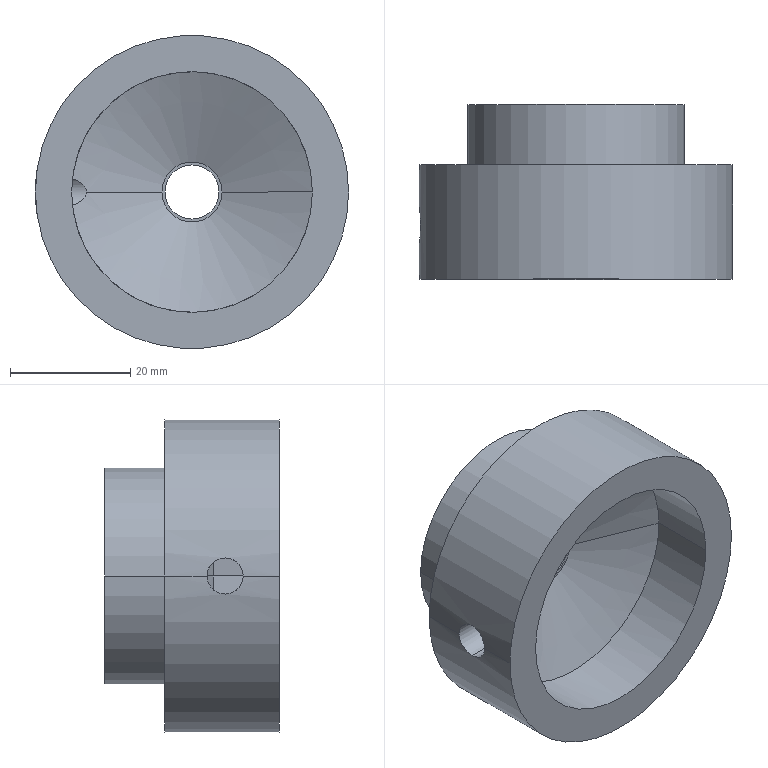Part | SolidWorks | features HoleWzd 1, ICE 1, Revolution 1 | 1 solid | 16 faces | box 52 x 29 x 52 mm | volume 32471 mm3 | cylinder 10 | plane 4 | cone 2 | commonest cylinder face diameters 6 x2 9 x2 36 x2 40 x2 52 x2
STEP:
#1=CARTESIAN_POINT('',(-25.826,9.,3.));
#2=VERTEX_POINT('',#1);
#3=CARTESIAN_POINT('',(-26.,6.,0.));
#4=VERTEX_POINT('',#3);
#5=CARTESIAN_POINT('',(-25.826,9.,3.));
#6=CARTESIAN_POINT('',(-25.826,8.802,3.));
#7=CARTESIAN_POINT('',(-25.829,8.607,2.981));
#8=CARTESIAN_POINT('',(-25.837,8.223,2.904));
#9=CARTESIAN_POINT('',(-25.844,8.033,2.847));
#10=CARTESIAN_POINT('',(-25.86,7.67,2.696));
#11=CARTESIAN_POINT('',(-25.869,7.498,2.604));
#12=CARTESIAN_POINT('',(-25.89,7.172,2.387));
#13=CARTESIAN_POINT('',(-25.902,7.018,2.26));
#14=CARTESIAN_POINT('',(-25.925,6.741,1.984));
#15=CARTESIAN_POINT('',(-25.936,6.617,1.833));
#16=CARTESIAN_POINT('',(-25.957,6.398,1.506));
#17=CARTESIAN_POINT('',(-25.967,6.305,1.331));
#18=CARTESIAN_POINT('',(-25.982,6.155,0.9708));
#19=CARTESIAN_POINT('',(-25.989,6.097,0.7819));
#20=CARTESIAN_POINT('',(-25.998,6.019,0.3943));
#21=CARTESIAN_POINT('',(-26.,6.,0.1983));
#22=CARTESIAN_POINT('',(-26.,6.,0.));
#23=B_SPLINE_CURVE_WITH_KNOTS('',3,(#5,#6,#7,#8,#9,#10,#11,#12,#13,#14,#15,#16,#17,#18,#19,#20,#21,#22),.UNSPECIFIED.,.F.,.F.,(4,2,2,2,2,2,2,2,4),(0.01408,0.01467,0.01525,0.01584,0.01643,0.01701,0.0176,0.01819,0.01877),.UNSPECIFIED.);
#24=EDGE_CURVE('',#2,#4,#23,.T.);
#25=ORIENTED_EDGE('',*,*,#24,.F.);
#26=CARTESIAN_POINT('',(-19.774,9.,3.));
#27=VERTEX_POINT('',#26);
#28=CARTESIAN_POINT('',(-26.,9.,3.));
#29=DIRECTION('',(1.,0.,0.));
#30=VECTOR('',#29,1000.);
#31=LINE('',#28,#30);
#32=EDGE_CURVE('',#2,#27,#31,.T.);
#33=ORIENTED_EDGE('',*,*,#32,.T.);
#34=CARTESIAN_POINT('',(-20.,6.,0.));
#35=VERTEX_POINT('',#34);
#36=CARTESIAN_POINT('',(-20.,6.,0.));
#37=CARTESIAN_POINT('',(-20.,6.,0.197));
#38=CARTESIAN_POINT('',(-19.997,6.02,0.3952));
#39=CARTESIAN_POINT('',(-19.986,6.096,0.779));
#40=CARTESIAN_POINT('',(-19.977,6.153,0.967));
#41=CARTESIAN_POINT('',(-19.956,6.305,1.333));
#42=CARTESIAN_POINT('',(-19.944,6.398,1.505));
#43=CARTESIAN_POINT('',(-19.917,6.615,1.83));
#44=CARTESIAN_POINT('',(-19.902,6.741,1.984));
#45=CARTESIAN_POINT('',(-19.872,7.019,2.261));
#46=CARTESIAN_POINT('',(-19.858,7.169,2.385));
#47=CARTESIAN_POINT('',(-19.83,7.495,2.603));
#48=CARTESIAN_POINT('',(-19.817,7.671,2.697));
#49=CARTESIAN_POINT('',(-19.797,8.033,2.846));
#50=CARTESIAN_POINT('',(-19.788,8.22,2.904));
#51=CARTESIAN_POINT('',(-19.777,8.608,2.981));
#52=CARTESIAN_POINT('',(-19.774,8.804,3.));
#53=CARTESIAN_POINT('',(-19.774,9.,3.));
#54=B_SPLINE_CURVE_WITH_KNOTS('',3,(#36,#37,#38,#39,#40,#41,#42,#43,#44,#45,#46,#47,#48,#49,#50,#51,#52,#53),.UNSPECIFIED.,.F.,.F.,(4,2,2,2,2,2,2,2,4),(0.00688,0.007467,0.008054,0.008641,0.009228,0.009815,0.0104,0.01099,0.01158),.UNSPECIFIED.);
#55=EDGE_CURVE('',#35,#27,#54,.T.);
#56=ORIENTED_EDGE('',*,*,#55,.F.);
#57=CARTESIAN_POINT('',(-19.774,9.,-3.));
#58=VERTEX_POINT('',#57);
#59=CARTESIAN_POINT('',(-19.774,9.,-3.));
#60=CARTESIAN_POINT('',(-19.774,8.803,-3.));
#61=CARTESIAN_POINT('',(-19.777,8.608,-2.981));
#62=CARTESIAN_POINT('',(-19.788,8.223,-2.904));
#63=CARTESIAN_POINT('',(-19.797,8.032,-2.846));
#64=CARTESIAN_POINT('',(-19.818,7.67,-2.696));
#65=CARTESIAN_POINT('',(-19.83,7.497,-2.604));
#66=CARTESIAN_POINT('',(-19.858,7.169,-2.385));
#67=CARTESIAN_POINT('',(-19.872,7.017,-2.259));
#68=CARTESIAN_POINT('',(-19.902,6.741,-1.983));
#69=CARTESIAN_POINT('',(-19.917,6.615,-1.83));
#70=CARTESIAN_POINT('',(-19.944,6.396,-1.503));
#71=CARTESIAN_POINT('',(-19.957,6.304,-1.33));
#72=CARTESIAN_POINT('',(-19.977,6.154,-0.9683));
#73=CARTESIAN_POINT('',(-19.986,6.096,-0.7769));
#74=CARTESIAN_POINT('',(-19.997,6.019,-0.3919));
#75=CARTESIAN_POINT('',(-20.,6.,-0.1971));
#76=CARTESIAN_POINT('',(-20.,6.,0.));
#77=B_SPLINE_CURVE_WITH_KNOTS('',3,(#59,#60,#61,#62,#63,#64,#65,#66,#67,#68,#69,#70,#71,#72,#73,#74,#75,#76),.UNSPECIFIED.,.F.,.F.,(4,2,2,2,2,2,2,2,4),(0.002181,0.002768,0.003356,0.003943,0.00453,0.005118,0.005705,0.006292,0.00688),.UNSPECIFIED.);
#78=EDGE_CURVE('',#58,#35,#77,.T.);
#79=ORIENTED_EDGE('',*,*,#78,.F.);
#80=CARTESIAN_POINT('',(-25.826,9.,-3.));
#81=VERTEX_POINT('',#80);
#82=CARTESIAN_POINT('',(-26.,9.,-3.));
#83=DIRECTION('',(1.,0.,0.));
#84=VECTOR('',#83,1000.);
#85=LINE('',#82,#84);
#86=EDGE_CURVE('',#81,#58,#85,.T.);
#87=ORIENTED_EDGE('',*,*,#86,.F.);
#88=CARTESIAN_POINT('',(-26.,6.,0.));
#89=CARTESIAN_POINT('',(-26.,6.,-0.1984));
#90=CARTESIAN_POINT('',(-25.998,6.019,-0.3935));
#91=CARTESIAN_POINT('',(-25.989,6.096,-0.7773));
#92=CARTESIAN_POINT('',(-25.983,6.154,-0.968));
#93=CARTESIAN_POINT('',(-25.967,6.304,-1.331));
#94=CARTESIAN_POINT('',(-25.957,6.397,-1.504));
#95=CARTESIAN_POINT('',(-25.936,6.614,-1.83));
#96=CARTESIAN_POINT('',(-25.925,6.741,-1.984));
#97=CARTESIAN_POINT('',(-25.902,7.018,-2.26));
#98=CARTESIAN_POINT('',(-25.891,7.169,-2.384));
#99=CARTESIAN_POINT('',(-25.87,7.497,-2.604));
#100=CARTESIAN_POINT('',(-25.86,7.671,-2.697));
#101=CARTESIAN_POINT('',(-25.844,8.032,-2.846));
#102=CARTESIAN_POINT('',(-25.837,8.222,-2.904));
#103=CARTESIAN_POINT('',(-25.829,8.609,-2.981));
#104=CARTESIAN_POINT('',(-25.826,8.804,-3.));
#105=CARTESIAN_POINT('',(-25.826,9.,-3.));
#106=B_SPLINE_CURVE_WITH_KNOTS('',3,(#88,#89,#90,#91,#92,#93,#94,#95,#96,#97,#98,#99,#100,#101,#102,#103,#104,#105),.UNSPECIFIED.,.F.,.F.,(4,2,2,2,2,2,2,2,4),(0.,0.0005868,0.001174,0.001761,0.002347,0.002934,0.003521,0.004108,0.004695),.UNSPECIFIED.);
#107=EDGE_CURVE('',#4,#81,#106,.T.);
#108=ORIENTED_EDGE('',*,*,#107,.F.);
#109=EDGE_LOOP('',(#25,#33,#56,#79,#87,#108));
#110=FACE_OUTER_BOUND('',#109,.T.);
#111=CARTESIAN_POINT('',(-26.,9.,0.));
#112=DIRECTION('',(1.,0.,0.));
#113=DIRECTION('',(0.,0.,-1.));
#114=AXIS2_PLACEMENT_3D('',#111,#112,#113);
#115=CYLINDRICAL_SURFACE('',#114,3.);
#116=ADVANCED_FACE('',(#110),#115,.F.);
#117=CARTESIAN_POINT('',(0.,17.,-4.5));
#118=VERTEX_POINT('',#117);
#119=CARTESIAN_POINT('',(0.,17.,4.5));
#120=VERTEX_POINT('',#119);
#121=CARTESIAN_POINT('',(0.,17.,0.));
#122=DIRECTION('',(0.,1.,0.));
#123=DIRECTION('',(-1.,0.,0.));
#124=AXIS2_PLACEMENT_3D('',#121,#122,#123);
#125=CIRCLE('',#124,4.5);
#126=EDGE_CURVE('',#118,#120,#125,.T.);
#127=ORIENTED_EDGE('',*,*,#126,.F.);
#128=CARTESIAN_POINT('',(0.,29.,-4.5));
#129=VERTEX_POINT('',#128);
#130=CARTESIAN_POINT('',(0.,29.,-4.5));
#131=DIRECTION('',(0.,1.,0.));
#132=VECTOR('',#131,1000.);
#133=LINE('',#130,#132);
#134=EDGE_CURVE('',#118,#129,#133,.T.);
#135=ORIENTED_EDGE('',*,*,#134,.T.);
#136=CARTESIAN_POINT('',(0.,29.,4.5));
#137=VERTEX_POINT('',#136);
#138=CARTESIAN_POINT('',(0.,29.,0.));
#139=DIRECTION('',(0.,1.,0.));
#140=DIRECTION('',(0.,0.,1.));
#141=AXIS2_PLACEMENT_3D('',#138,#139,#140);
#142=CIRCLE('',#141,4.5);
#143=EDGE_CURVE('',#129,#137,#142,.T.);
#144=ORIENTED_EDGE('',*,*,#143,.T.);
#145=CARTESIAN_POINT('',(0.,29.,4.5));
#146=DIRECTION('',(0.,1.,0.));
#147=VECTOR('',#146,1000.);
#148=LINE('',#145,#147);
#149=EDGE_CURVE('',#120,#137,#148,.T.);
#150=ORIENTED_EDGE('',*,*,#149,.F.);
#151=EDGE_LOOP('',(#127,#135,#144,#150));
#152=FACE_OUTER_BOUND('',#151,.T.);
#153=CARTESIAN_POINT('',(0.,29.,0.));
#154=DIRECTION('',(0.,1.,0.));
#155=DIRECTION('',(0.,0.,1.));
#156=AXIS2_PLACEMENT_3D('',#153,#154,#155);
#157=CYLINDRICAL_SURFACE('',#156,4.5);
#158=ADVANCED_FACE('',(#152),#157,.F.);
#159=CARTESIAN_POINT('',(-18.,19.,0.));
#160=VERTEX_POINT('',#159);
#161=CARTESIAN_POINT('',(18.,19.,0.));
#162=VERTEX_POINT('',#161);
#163=CARTESIAN_POINT('',(0.,19.,0.));
#164=DIRECTION('',(0.,1.,0.));
#165=DIRECTION('',(-1.,0.,0.));
#166=AXIS2_PLACEMENT_3D('',#163,#164,#165);
#167=CIRCLE('',#166,18.);
#168=EDGE_CURVE('',#160,#162,#167,.T.);
#169=ORIENTED_EDGE('',*,*,#168,.T.);
#170=CARTESIAN_POINT('',(18.,29.,0.));
#171=VERTEX_POINT('',#170);
#172=CARTESIAN_POINT('',(18.,29.712,0.));
#173=DIRECTION('',(0.,1.,0.));
#174=VECTOR('',#173,1000.);
#175=LINE('',#172,#174);
#176=EDGE_CURVE('',#162,#171,#175,.T.);
#177=ORIENTED_EDGE('',*,*,#176,.T.);
#178=CARTESIAN_POINT('',(-18.,29.,0.));
#179=VERTEX_POINT('',#178);
#180=CARTESIAN_POINT('',(0.,29.,0.));
#181=DIRECTION('',(0.,1.,0.));
#182=DIRECTION('',(-1.,0.,0.));
#183=AXIS2_PLACEMENT_3D('',#180,#181,#182);
#184=CIRCLE('',#183,18.);
#185=EDGE_CURVE('',#179,#171,#184,.T.);
#186=ORIENTED_EDGE('',*,*,#185,.F.);
#187=CARTESIAN_POINT('',(-18.,29.712,0.));
#188=DIRECTION('',(0.,1.,0.));
#189=VECTOR('',#188,1000.);
#190=LINE('',#187,#189);
#191=EDGE_CURVE('',#160,#179,#190,.T.);
#192=ORIENTED_EDGE('',*,*,#191,.F.);
#193=EDGE_LOOP('',(#169,#177,#186,#192));
#194=FACE_OUTER_BOUND('',#193,.T.);
#195=CARTESIAN_POINT('',(0.,29.712,0.));
#196=DIRECTION('',(0.,1.,0.));
#197=DIRECTION('',(-1.,0.,0.));
#198=AXIS2_PLACEMENT_3D('',#195,#196,#197);
#199=CYLINDRICAL_SURFACE('',#198,18.);
#200=ADVANCED_FACE('',(#194),#199,.T.);
#201=CARTESIAN_POINT('',(5.,17.,0.));
#202=VERTEX_POINT('',#201);
#203=CARTESIAN_POINT('',(-5.,17.,0.));
#204=VERTEX_POINT('',#203);
#205=CARTESIAN_POINT('',(0.,17.,0.));
#206=DIRECTION('',(0.,1.,0.));
#207=DIRECTION('',(-1.,0.,0.));
#208=AXIS2_PLACEMENT_3D('',#205,#206,#207);
#209=CIRCLE('',#208,5.);
#210=EDGE_CURVE('',#202,#204,#209,.T.);
#211=ORIENTED_EDGE('',*,*,#210,.T.);
#212=CARTESIAN_POINT('',(-17.5,12.,0.));
#213=VERTEX_POINT('',#212);
#214=CARTESIAN_POINT('',(-5.,17.,0.));
#215=DIRECTION('',(-0.9285,-0.3714,0.));
#216=VECTOR('',#215,1000.);
#217=LINE('',#214,#216);
#218=EDGE_CURVE('',#204,#213,#217,.T.);
#219=ORIENTED_EDGE('',*,*,#218,.T.);
#220=CARTESIAN_POINT('',(-19.875,11.,-2.236));
#221=VERTEX_POINT('',#220);
#222=CARTESIAN_POINT('',(-17.5,12.,0.));
#223=CARTESIAN_POINT('',(-17.5,12.,-0.1503));
#224=CARTESIAN_POINT('',(-17.528,11.988,-0.302));
#225=CARTESIAN_POINT('',(-17.626,11.946,-0.5843));
#226=CARTESIAN_POINT('',(-17.697,11.916,-0.7175));
#227=CARTESIAN_POINT('',(-17.944,11.81,-1.08));
#228=CARTESIAN_POINT('',(-18.157,11.72,-1.282));
#229=CARTESIAN_POINT('',(-18.608,11.529,-1.626));
#230=CARTESIAN_POINT('',(-18.851,11.427,-1.772));
#231=CARTESIAN_POINT('',(-19.353,11.216,-2.029));
#232=CARTESIAN_POINT('',(-19.612,11.109,-2.139));
#233=CARTESIAN_POINT('',(-19.875,11.,-2.236));
#234=B_SPLINE_CURVE_WITH_KNOTS('',3,(#222,#223,#224,#225,#226,#227,#228,#229,#230,#231,#232,#233),.UNSPECIFIED.,.F.,.F.,(4,2,2,2,2,4),(0.003869,0.004318,0.004766,0.005664,0.006561,0.007459),.UNSPECIFIED.);
#235=EDGE_CURVE('',#213,#221,#234,.T.);
#236=ORIENTED_EDGE('',*,*,#235,.T.);
#237=CARTESIAN_POINT('',(20.,11.,0.));
#238=VERTEX_POINT('',#237);
#239=CARTESIAN_POINT('',(0.,11.,0.));
#240=DIRECTION('',(0.,1.,0.));
#241=DIRECTION('',(-1.,0.,0.));
#242=AXIS2_PLACEMENT_3D('',#239,#240,#241);
#243=CIRCLE('',#242,20.);
#244=EDGE_CURVE('',#238,#221,#243,.T.);
#245=ORIENTED_EDGE('',*,*,#244,.F.);
#246=CARTESIAN_POINT('',(5.,17.,0.));
#247=DIRECTION('',(0.9285,-0.3714,0.));
#248=VECTOR('',#247,1000.);
#249=LINE('',#246,#248);
#250=EDGE_CURVE('',#202,#238,#249,.T.);
#251=ORIENTED_EDGE('',*,*,#250,.F.);
#252=EDGE_LOOP('',(#211,#219,#236,#245,#251));
#253=FACE_OUTER_BOUND('',#252,.T.);
#254=CARTESIAN_POINT('',(0.,17.,0.));
#255=DIRECTION('',(0.,-1.,0.));
#256=DIRECTION('',(1.,0.,0.));
#257=AXIS2_PLACEMENT_3D('',#254,#255,#256);
#258=CONICAL_SURFACE('',#257,5.,1.19);
#259=ADVANCED_FACE('',(#253),#258,.F.);
#260=CARTESIAN_POINT('',(20.,0.,0.));
#261=VERTEX_POINT('',#260);
#262=CARTESIAN_POINT('',(-20.,0.,0.));
#263=VERTEX_POINT('',#262);
#264=CARTESIAN_POINT('',(0.,0.,0.));
#265=DIRECTION('',(0.,1.,0.));
#266=DIRECTION('',(-1.,0.,0.));
#267=AXIS2_PLACEMENT_3D('',#264,#265,#266);
#268=CIRCLE('',#267,20.);
#269=EDGE_CURVE('',#261,#263,#268,.T.);
#270=ORIENTED_EDGE('',*,*,#269,.F.);
#271=CARTESIAN_POINT('',(20.,29.712,0.));
#272=DIRECTION('',(0.,1.,0.));
#273=VECTOR('',#272,1000.);
#274=LINE('',#271,#273);
#275=EDGE_CURVE('',#261,#238,#274,.T.);
#276=ORIENTED_EDGE('',*,*,#275,.T.);
#277=ORIENTED_EDGE('',*,*,#244,.T.);
#278=CARTESIAN_POINT('',(-19.875,11.,-2.236));
#279=CARTESIAN_POINT('',(-19.861,10.863,-2.359));
#280=CARTESIAN_POINT('',(-19.848,10.717,-2.467));
#281=CARTESIAN_POINT('',(-19.823,10.407,-2.656));
#282=CARTESIAN_POINT('',(-19.812,10.242,-2.737));
#283=CARTESIAN_POINT('',(-19.793,9.9,-2.868));
#284=CARTESIAN_POINT('',(-19.786,9.725,-2.917));
#285=CARTESIAN_POINT('',(-19.776,9.367,-2.983));
#286=CARTESIAN_POINT('',(-19.774,9.183,-3.));
#287=CARTESIAN_POINT('',(-19.774,9.,-3.));
#288=B_SPLINE_CURVE_WITH_KNOTS('',3,(#278,#279,#280,#281,#282,#283,#284,#285,#286,#287),.UNSPECIFIED.,.F.,.F.,(4,2,2,2,4),(0.,0.0005452,0.00109,0.001636,0.002181),.UNSPECIFIED.);
#289=EDGE_CURVE('',#221,#58,#288,.T.);
#290=ORIENTED_EDGE('',*,*,#289,.T.);
#291=ORIENTED_EDGE('',*,*,#78,.T.);
#292=CARTESIAN_POINT('',(-20.,29.712,0.));
#293=DIRECTION('',(0.,1.,0.));
#294=VECTOR('',#293,1000.);
#295=LINE('',#292,#294);
#296=EDGE_CURVE('',#263,#35,#295,.T.);
#297=ORIENTED_EDGE('',*,*,#296,.F.);
#298=EDGE_LOOP('',(#270,#276,#277,#290,#291,#297));
#299=FACE_OUTER_BOUND('',#298,.T.);
#300=CARTESIAN_POINT('',(0.,29.712,0.));
#301=DIRECTION('',(0.,1.,0.));
#302=DIRECTION('',(-1.,0.,0.));
#303=AXIS2_PLACEMENT_3D('',#300,#301,#302);
#304=CYLINDRICAL_SURFACE('',#303,20.);
#305=ADVANCED_FACE('',(#299),#304,.F.);
#306=CARTESIAN_POINT('',(-26.,0.,0.));
#307=VERTEX_POINT('',#306);
#308=CARTESIAN_POINT('',(26.,0.,0.));
#309=VERTEX_POINT('',#308);
#310=CARTESIAN_POINT('',(0.,0.,0.));
#311=DIRECTION('',(0.,1.,0.));
#312=DIRECTION('',(-1.,0.,0.));
#313=AXIS2_PLACEMENT_3D('',#310,#311,#312);
#314=CIRCLE('',#313,26.);
#315=EDGE_CURVE('',#307,#309,#314,.T.);
#316=ORIENTED_EDGE('',*,*,#315,.T.);
#317=CARTESIAN_POINT('',(26.,19.,0.));
#318=VERTEX_POINT('',#317);
#319=CARTESIAN_POINT('',(26.,29.712,0.));
#320=DIRECTION('',(0.,1.,0.));
#321=VECTOR('',#320,1000.);
#322=LINE('',#319,#321);
#323=EDGE_CURVE('',#309,#318,#322,.T.);
#324=ORIENTED_EDGE('',*,*,#323,.T.);
#325=CARTESIAN_POINT('',(-26.,19.,0.));
#326=VERTEX_POINT('',#325);
#327=CARTESIAN_POINT('',(0.,19.,0.));
#328=DIRECTION('',(0.,1.,0.));
#329=DIRECTION('',(-1.,0.,0.));
#330=AXIS2_PLACEMENT_3D('',#327,#328,#329);
#331=CIRCLE('',#330,26.);
#332=EDGE_CURVE('',#326,#318,#331,.T.);
#333=ORIENTED_EDGE('',*,*,#332,.F.);
#334=CARTESIAN_POINT('',(-26.,12.,0.));
#335=VERTEX_POINT('',#334);
#336=CARTESIAN_POINT('',(-26.,29.712,0.));
#337=DIRECTION('',(0.,1.,0.));
#338=VECTOR('',#337,1000.);
#339=LINE('',#336,#338);
#340=EDGE_CURVE('',#335,#326,#339,.T.);
#341=ORIENTED_EDGE('',*,*,#340,.F.);
#342=CARTESIAN_POINT('',(-26.,12.,0.));
#343=CARTESIAN_POINT('',(-26.,12.,0.1959));
#344=CARTESIAN_POINT('',(-25.998,11.981,0.3908));
#345=CARTESIAN_POINT('',(-25.989,11.904,0.7782));
#346=CARTESIAN_POINT('',(-25.983,11.846,0.9676));
#347=CARTESIAN_POINT('',(-25.967,11.697,1.329));
#348=CARTESIAN_POINT('',(-25.957,11.604,1.503));
#349=CARTESIAN_POINT('',(-25.936,11.384,1.831));
#350=CARTESIAN_POINT('',(-25.925,11.26,1.982));
#351=CARTESIAN_POINT('',(-25.902,10.984,2.259));
#352=CARTESIAN_POINT('',(-25.891,10.829,2.386));
#353=CARTESIAN_POINT('',(-25.87,10.503,2.603));
#354=CARTESIAN_POINT('',(-25.86,10.331,2.696));
#355=CARTESIAN_POINT('',(-25.844,9.968,2.846));
#356=CARTESIAN_POINT('',(-25.837,9.777,2.904));
#357=CARTESIAN_POINT('',(-25.829,9.394,2.981));
#358=CARTESIAN_POINT('',(-25.826,9.198,3.));
#359=CARTESIAN_POINT('',(-25.826,9.,3.));
#360=B_SPLINE_CURVE_WITH_KNOTS('',3,(#342,#343,#344,#345,#346,#347,#348,#349,#350,#351,#352,#353,#354,#355,#356,#357,#358,#359),.UNSPECIFIED.,.F.,.F.,(4,2,2,2,2,2,2,2,4),(0.009387,0.009974,0.01056,0.01115,0.01173,0.01232,0.01291,0.0135,0.01408),.UNSPECIFIED.);
#361=EDGE_CURVE('',#335,#2,#360,.T.);
#362=ORIENTED_EDGE('',*,*,#361,.T.);
#363=ORIENTED_EDGE('',*,*,#24,.T.);
#364=CARTESIAN_POINT('',(-26.,29.712,0.));
#365=DIRECTION('',(0.,1.,0.));
#366=VECTOR('',#365,1000.);
#367=LINE('',#364,#366);
#368=EDGE_CURVE('',#307,#4,#367,.T.);
#369=ORIENTED_EDGE('',*,*,#368,.F.);
#370=EDGE_LOOP('',(#316,#324,#333,#341,#362,#363,#369));
#371=FACE_OUTER_BOUND('',#370,.T.);
#372=CARTESIAN_POINT('',(0.,29.712,0.));
#373=DIRECTION('',(0.,1.,0.));
#374=DIRECTION('',(-1.,0.,0.));
#375=AXIS2_PLACEMENT_3D('',#372,#373,#374);
#376=CYLINDRICAL_SURFACE('',#375,26.);
#377=ADVANCED_FACE('',(#371),#376,.T.);
#378=ORIENTED_EDGE('',*,*,#185,.T.);
#379=CARTESIAN_POINT('',(0.,29.,0.));
#380=DIRECTION('',(0.,1.,0.));
#381=DIRECTION('',(-1.,0.,0.));
#382=AXIS2_PLACEMENT_3D('',#379,#380,#381);
#383=CIRCLE('',#382,18.);
#384=EDGE_CURVE('',#171,#179,#383,.T.);
#385=ORIENTED_EDGE('',*,*,#384,.T.);
#386=EDGE_LOOP('',(#378,#385));
#387=FACE_OUTER_BOUND('',#386,.T.);
#388=CARTESIAN_POINT('',(0.,29.,0.));
#389=DIRECTION('',(0.,1.,0.));
#390=DIRECTION('',(0.,0.,1.));
#391=AXIS2_PLACEMENT_3D('',#388,#389,#390);
#392=CIRCLE('',#391,4.5);
#393=EDGE_CURVE('',#137,#129,#392,.T.);
#394=ORIENTED_EDGE('',*,*,#393,.F.);
#395=ORIENTED_EDGE('',*,*,#143,.F.);
#396=EDGE_LOOP('',(#394,#395));
#397=FACE_BOUND('',#396,.T.);
#398=CARTESIAN_POINT('',(18.,29.,0.));
#399=DIRECTION('',(0.,-1.,0.));
#400=DIRECTION('',(1.,0.,0.));
#401=AXIS2_PLACEMENT_3D('',#398,#399,#400);
#402=PLANE('',#401);
#403=ADVANCED_FACE('',(#387,#397),#402,.F.);
#404=ORIENTED_EDGE('',*,*,#168,.F.);
#405=CARTESIAN_POINT('',(0.,19.,0.));
#406=DIRECTION('',(0.,1.,0.));
#407=DIRECTION('',(-1.,0.,0.));
#408=AXIS2_PLACEMENT_3D('',#405,#406,#407);
#409=CIRCLE('',#408,18.);
#410=EDGE_CURVE('',#162,#160,#409,.T.);
#411=ORIENTED_EDGE('',*,*,#410,.F.);
#412=EDGE_LOOP('',(#404,#411));
#413=FACE_BOUND('',#412,.T.);
#414=ORIENTED_EDGE('',*,*,#332,.T.);
#415=CARTESIAN_POINT('',(0.,19.,0.));
#416=DIRECTION('',(0.,1.,0.));
#417=DIRECTION('',(-1.,0.,0.));
#418=AXIS2_PLACEMENT_3D('',#415,#416,#417);
#419=CIRCLE('',#418,26.);
#420=EDGE_CURVE('',#318,#326,#419,.T.);
#421=ORIENTED_EDGE('',*,*,#420,.T.);
#422=EDGE_LOOP('',(#414,#421));
#423=FACE_OUTER_BOUND('',#422,.T.);
#424=CARTESIAN_POINT('',(26.,19.,0.));
#425=DIRECTION('',(0.,-1.,0.));
#426=DIRECTION('',(1.,0.,0.));
#427=AXIS2_PLACEMENT_3D('',#424,#425,#426);
#428=PLANE('',#427);
#429=ADVANCED_FACE('',(#413,#423),#428,.F.);
#430=ORIENTED_EDGE('',*,*,#323,.F.);
#431=CARTESIAN_POINT('',(0.,0.,0.));
#432=DIRECTION('',(0.,1.,0.));
#433=DIRECTION('',(-1.,0.,0.));
#434=AXIS2_PLACEMENT_3D('',#431,#432,#433);
#435=CIRCLE('',#434,26.);
#436=EDGE_CURVE('',#309,#307,#435,.T.);
#437=ORIENTED_EDGE('',*,*,#436,.T.);
#438=ORIENTED_EDGE('',*,*,#368,.T.);
#439=ORIENTED_EDGE('',*,*,#107,.T.);
#440=CARTESIAN_POINT('',(-25.826,9.,-3.));
#441=CARTESIAN_POINT('',(-25.826,9.196,-3.));
#442=CARTESIAN_POINT('',(-25.829,9.395,-2.98));
#443=CARTESIAN_POINT('',(-25.837,9.779,-2.904));
#444=CARTESIAN_POINT('',(-25.844,9.967,-2.847));
#445=CARTESIAN_POINT('',(-25.86,10.33,-2.696));
#446=CARTESIAN_POINT('',(-25.87,10.505,-2.602));
#447=CARTESIAN_POINT('',(-25.891,10.83,-2.385));
#448=CARTESIAN_POINT('',(-25.902,10.981,-2.261));
#449=CARTESIAN_POINT('',(-25.925,11.261,-1.981));
#450=CARTESIAN_POINT('',(-25.936,11.385,-1.83));
#451=CARTESIAN_POINT('',(-25.957,11.602,-1.505));
#452=CARTESIAN_POINT('',(-25.967,11.696,-1.33));
#453=CARTESIAN_POINT('',(-25.983,11.847,-0.9664));
#454=CARTESIAN_POINT('',(-25.989,11.904,-0.7795));
#455=CARTESIAN_POINT('',(-25.998,11.98,-0.3948));
#456=CARTESIAN_POINT('',(-26.,12.,-0.1958));
#457=CARTESIAN_POINT('',(-26.,12.,0.));
#458=B_SPLINE_CURVE_WITH_KNOTS('',3,(#440,#441,#442,#443,#444,#445,#446,#447,#448,#449,#450,#451,#452,#453,#454,#455,#456,#457),.UNSPECIFIED.,.F.,.F.,(4,2,2,2,2,2,2,2,4),(0.004695,0.005281,0.005868,0.006454,0.007041,0.007627,0.008214,0.008801,0.009387),.UNSPECIFIED.);
#459=EDGE_CURVE('',#81,#335,#458,.T.);
#460=ORIENTED_EDGE('',*,*,#459,.T.);
#461=ORIENTED_EDGE('',*,*,#340,.T.);
#462=ORIENTED_EDGE('',*,*,#420,.F.);
#463=EDGE_LOOP('',(#430,#437,#438,#439,#460,#461,#462));
#464=FACE_OUTER_BOUND('',#463,.T.);
#465=CARTESIAN_POINT('',(0.,29.712,0.));
#466=DIRECTION('',(0.,1.,0.));
#467=DIRECTION('',(-1.,0.,0.));
#468=AXIS2_PLACEMENT_3D('',#465,#466,#467);
#469=CYLINDRICAL_SURFACE('',#468,26.);
#470=ADVANCED_FACE('',(#464),#469,.T.);
#471=ORIENTED_EDGE('',*,*,#315,.F.);
#472=ORIENTED_EDGE('',*,*,#436,.F.);
#473=EDGE_LOOP('',(#471,#472));
#474=FACE_OUTER_BOUND('',#473,.T.);
#475=CARTESIAN_POINT('',(0.,0.,0.));
#476=DIRECTION('',(0.,1.,0.));
#477=DIRECTION('',(-1.,0.,0.));
#478=AXIS2_PLACEMENT_3D('',#475,#476,#477);
#479=CIRCLE('',#478,20.);
#480=EDGE_CURVE('',#263,#261,#479,.T.);
#481=ORIENTED_EDGE('',*,*,#480,.T.);
#482=ORIENTED_EDGE('',*,*,#269,.T.);
#483=EDGE_LOOP('',(#481,#482));
#484=FACE_BOUND('',#483,.T.);
#485=CARTESIAN_POINT('',(20.,0.,0.));
#486=DIRECTION('',(0.,1.,0.));
#487=DIRECTION('',(-1.,0.,0.));
#488=AXIS2_PLACEMENT_3D('',#485,#486,#487);
#489=PLANE('',#488);
#490=ADVANCED_FACE('',(#474,#484),#489,.F.);
#491=ORIENTED_EDGE('',*,*,#275,.F.);
#492=ORIENTED_EDGE('',*,*,#480,.F.);
#493=ORIENTED_EDGE('',*,*,#296,.T.);
#494=ORIENTED_EDGE('',*,*,#55,.T.);
#495=CARTESIAN_POINT('',(-19.875,11.,2.236));
#496=VERTEX_POINT('',#495);
#497=CARTESIAN_POINT('',(-19.774,9.,3.));
#498=CARTESIAN_POINT('',(-19.774,9.181,3.));
#499=CARTESIAN_POINT('',(-19.776,9.364,2.983));
#500=CARTESIAN_POINT('',(-19.786,9.725,2.917));
#501=CARTESIAN_POINT('',(-19.793,9.9,2.868));
#502=CARTESIAN_POINT('',(-19.812,10.239,2.738));
#503=CARTESIAN_POINT('',(-19.823,10.404,2.657));
#504=CARTESIAN_POINT('',(-19.847,10.717,2.467));
#505=CARTESIAN_POINT('',(-19.861,10.863,2.358));
#506=CARTESIAN_POINT('',(-19.875,11.,2.236));
#507=B_SPLINE_CURVE_WITH_KNOTS('',3,(#497,#498,#499,#500,#501,#502,#503,#504,#505,#506),.UNSPECIFIED.,.F.,.F.,(4,2,2,2,4),(0.01158,0.01212,0.01266,0.01321,0.01375),.UNSPECIFIED.);
#508=EDGE_CURVE('',#27,#496,#507,.T.);
#509=ORIENTED_EDGE('',*,*,#508,.T.);
#510=CARTESIAN_POINT('',(0.,11.,0.));
#511=DIRECTION('',(0.,1.,0.));
#512=DIRECTION('',(-1.,0.,0.));
#513=AXIS2_PLACEMENT_3D('',#510,#511,#512);
#514=CIRCLE('',#513,20.);
#515=EDGE_CURVE('',#496,#238,#514,.T.);
#516=ORIENTED_EDGE('',*,*,#515,.T.);
#517=EDGE_LOOP('',(#491,#492,#493,#494,#509,#516));
#518=FACE_OUTER_BOUND('',#517,.T.);
#519=CARTESIAN_POINT('',(0.,29.712,0.));
#520=DIRECTION('',(0.,1.,0.));
#521=DIRECTION('',(-1.,0.,0.));
#522=AXIS2_PLACEMENT_3D('',#519,#520,#521);
#523=CYLINDRICAL_SURFACE('',#522,20.);
#524=ADVANCED_FACE('',(#518),#523,.F.);
#525=ORIENTED_EDGE('',*,*,#218,.F.);
#526=CARTESIAN_POINT('',(0.,17.,0.));
#527=DIRECTION('',(0.,1.,0.));
#528=DIRECTION('',(-1.,0.,0.));
#529=AXIS2_PLACEMENT_3D('',#526,#527,#528);
#530=CIRCLE('',#529,5.);
#531=EDGE_CURVE('',#204,#202,#530,.T.);
#532=ORIENTED_EDGE('',*,*,#531,.T.);
#533=ORIENTED_EDGE('',*,*,#250,.T.);
#534=ORIENTED_EDGE('',*,*,#515,.F.);
#535=CARTESIAN_POINT('',(-19.875,11.,2.236));
#536=CARTESIAN_POINT('',(-19.612,11.109,2.139));
#537=CARTESIAN_POINT('',(-19.354,11.216,2.029));
#538=CARTESIAN_POINT('',(-18.854,11.425,1.774));
#539=CARTESIAN_POINT('',(-18.609,11.528,1.627));
#540=CARTESIAN_POINT('',(-18.155,11.72,1.281));
#541=CARTESIAN_POINT('',(-17.943,11.811,1.079));
#542=CARTESIAN_POINT('',(-17.697,11.916,0.7178));
#543=CARTESIAN_POINT('',(-17.626,11.946,0.5849));
#544=CARTESIAN_POINT('',(-17.528,11.988,0.3025));
#545=CARTESIAN_POINT('',(-17.5,12.,0.1505));
#546=CARTESIAN_POINT('',(-17.5,12.,0.));
#547=B_SPLINE_CURVE_WITH_KNOTS('',3,(#535,#536,#537,#538,#539,#540,#541,#542,#543,#544,#545,#546),.UNSPECIFIED.,.F.,.F.,(4,2,2,2,2,4),(0.0002747,0.001173,0.002072,0.00297,0.00342,0.003869),.UNSPECIFIED.);
#548=EDGE_CURVE('',#496,#213,#547,.T.);
#549=ORIENTED_EDGE('',*,*,#548,.T.);
#550=EDGE_LOOP('',(#525,#532,#533,#534,#549));
#551=FACE_OUTER_BOUND('',#550,.T.);
#552=CARTESIAN_POINT('',(0.,17.,0.));
#553=DIRECTION('',(0.,-1.,0.));
#554=DIRECTION('',(1.,0.,0.));
#555=AXIS2_PLACEMENT_3D('',#552,#553,#554);
#556=CONICAL_SURFACE('',#555,5.,1.19);
#557=ADVANCED_FACE('',(#551),#556,.F.);
#558=CARTESIAN_POINT('',(0.,17.,0.));
#559=DIRECTION('',(0.,1.,0.));
#560=DIRECTION('',(-1.,0.,0.));
#561=AXIS2_PLACEMENT_3D('',#558,#559,#560);
#562=CIRCLE('',#561,4.5);
#563=EDGE_CURVE('',#120,#118,#562,.T.);
#564=ORIENTED_EDGE('',*,*,#563,.T.);
#565=ORIENTED_EDGE('',*,*,#126,.T.);
#566=EDGE_LOOP('',(#564,#565));
#567=FACE_BOUND('',#566,.T.);
#568=ORIENTED_EDGE('',*,*,#210,.F.);
#569=ORIENTED_EDGE('',*,*,#531,.F.);
#570=EDGE_LOOP('',(#568,#569));
#571=FACE_OUTER_BOUND('',#570,.T.);
#572=CARTESIAN_POINT('',(5.,17.,0.));
#573=DIRECTION('',(0.,1.,0.));
#574=DIRECTION('',(-1.,0.,0.));
#575=AXIS2_PLACEMENT_3D('',#572,#573,#574);
#576=PLANE('',#575);
#577=ADVANCED_FACE('',(#567,#571),#576,.F.);
#578=ORIENTED_EDGE('',*,*,#176,.F.);
#579=ORIENTED_EDGE('',*,*,#410,.T.);
#580=ORIENTED_EDGE('',*,*,#191,.T.);
#581=ORIENTED_EDGE('',*,*,#384,.F.);
#582=EDGE_LOOP('',(#578,#579,#580,#581));
#583=FACE_OUTER_BOUND('',#582,.T.);
#584=CARTESIAN_POINT('',(0.,29.712,0.));
#585=DIRECTION('',(0.,1.,0.));
#586=DIRECTION('',(-1.,0.,0.));
#587=AXIS2_PLACEMENT_3D('',#584,#585,#586);
#588=CYLINDRICAL_SURFACE('',#587,18.);
#589=ADVANCED_FACE('',(#583),#588,.T.);
#590=ORIENTED_EDGE('',*,*,#134,.F.);
#591=ORIENTED_EDGE('',*,*,#563,.F.);
#592=ORIENTED_EDGE('',*,*,#149,.T.);
#593=ORIENTED_EDGE('',*,*,#393,.T.);
#594=EDGE_LOOP('',(#590,#591,#592,#593));
#595=FACE_OUTER_BOUND('',#594,.T.);
#596=CARTESIAN_POINT('',(0.,29.,0.));
#597=DIRECTION('',(0.,1.,0.));
#598=DIRECTION('',(0.,0.,1.));
#599=AXIS2_PLACEMENT_3D('',#596,#597,#598);
#600=CYLINDRICAL_SURFACE('',#599,4.5);
#601=ADVANCED_FACE('',(#595),#600,.F.);
#602=ORIENTED_EDGE('',*,*,#32,.F.);
#603=ORIENTED_EDGE('',*,*,#361,.F.);
#604=ORIENTED_EDGE('',*,*,#459,.F.);
#605=ORIENTED_EDGE('',*,*,#86,.T.);
#606=ORIENTED_EDGE('',*,*,#289,.F.);
#607=ORIENTED_EDGE('',*,*,#235,.F.);
#608=ORIENTED_EDGE('',*,*,#548,.F.);
#609=ORIENTED_EDGE('',*,*,#508,.F.);
#610=EDGE_LOOP('',(#602,#603,#604,#605,#606,#607,#608,#609));
#611=FACE_OUTER_BOUND('',#610,.T.);
#612=CARTESIAN_POINT('',(-26.,9.,0.));
#613=DIRECTION('',(1.,0.,0.));
#614=DIRECTION('',(0.,0.,-1.));
#615=AXIS2_PLACEMENT_3D('',#612,#613,#614);
#616=CYLINDRICAL_SURFACE('',#615,3.);
#617=ADVANCED_FACE('',(#611),#616,.F.);
#618=CLOSED_SHELL('',(#116,#158,#200,#259,#305,#377,#403,#429,#470,#490,#524,#557,#577,#589,#601,#617));
#619=MANIFOLD_SOLID_BREP('',#618);
#620=CARTESIAN_POINT('',(0.,0.,0.));
#621=DIRECTION('',(0.,0.,1.));
#622=DIRECTION('',(1.,0.,0.));
#623=AXIS2_PLACEMENT_3D('',#620,#621,#622);
#624=(LENGTH_UNIT()NAMED_UNIT(*)SI_UNIT(.MILLI.,.METRE.));
#625=UNCERTAINTY_MEASURE_WITH_UNIT(LENGTH_MEASURE(0.00001),#624,'','');
#626=(NAMED_UNIT(*)PLANE_ANGLE_UNIT()SI_UNIT($,.RADIAN.));
#627=(NAMED_UNIT(*)SI_UNIT($,.STERADIAN.)SOLID_ANGLE_UNIT());
#628=(GEOMETRIC_REPRESENTATION_CONTEXT(3)GLOBAL_UNCERTAINTY_ASSIGNED_CONTEXT((#625))GLOBAL_UNIT_ASSIGNED_CONTEXT((#624,#626,#627))REPRESENTATION_CONTEXT('',''));
#629=ADVANCED_BREP_SHAPE_REPRESENTATION('',(#619,#623),#628);